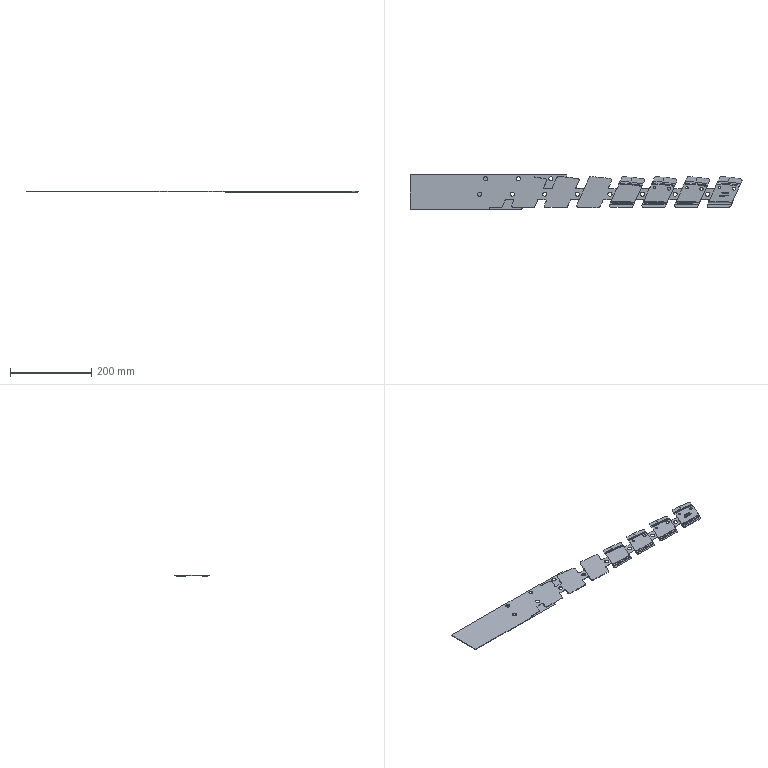Part | CATIA | 3 solids | 495 faces | volume 50816 mm3 | plane 277 | spline 114 | cylinder 100 | other 4 | commonest cylinder face diameters 6 x29 40 x28 10.2 x14 8 x10 15788 x7 25439 x4